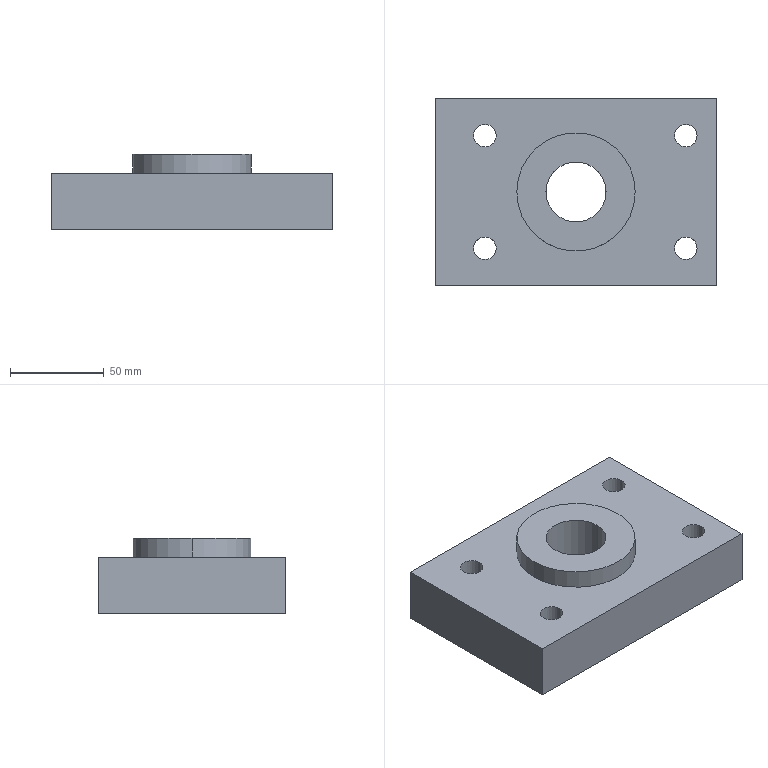Part | SolidWorks | features ICE 3, Extrusion 1 | 1 solid | 19 faces | box 150 x 100 x 40 mm | volume 435431 mm3 | cylinder 12 | plane 7 | commonest cylinder face diameters 12 x8 32 x2 63 x2
STEP:
#1=CARTESIAN_POINT('',(64.5,-30.,30.));
#2=VERTEX_POINT('',#1);
#3=CARTESIAN_POINT('',(52.5,-30.,30.));
#4=VERTEX_POINT('',#3);
#5=CARTESIAN_POINT('',(58.5,-30.,30.));
#6=DIRECTION('',(0.,0.,-1.));
#7=DIRECTION('',(-1.,0.,0.));
#8=AXIS2_PLACEMENT_3D('',#5,#6,#7);
#9=CIRCLE('',#8,6.);
#10=EDGE_CURVE('',#2,#4,#9,.T.);
#11=ORIENTED_EDGE('',*,*,#10,.F.);
#12=CARTESIAN_POINT('',(64.5,-30.,0.));
#13=VERTEX_POINT('',#12);
#14=CARTESIAN_POINT('',(64.5,-30.,40.));
#15=DIRECTION('',(0.,0.,-1.));
#16=VECTOR('',#15,1000.);
#17=LINE('',#14,#16);
#18=EDGE_CURVE('',#2,#13,#17,.T.);
#19=ORIENTED_EDGE('',*,*,#18,.T.);
#20=CARTESIAN_POINT('',(52.5,-30.,0.));
#21=VERTEX_POINT('',#20);
#22=CARTESIAN_POINT('',(58.5,-30.,0.));
#23=DIRECTION('',(0.,0.,-1.));
#24=DIRECTION('',(-1.,0.,0.));
#25=AXIS2_PLACEMENT_3D('',#22,#23,#24);
#26=CIRCLE('',#25,6.);
#27=EDGE_CURVE('',#13,#21,#26,.T.);
#28=ORIENTED_EDGE('',*,*,#27,.T.);
#29=CARTESIAN_POINT('',(52.5,-30.,40.));
#30=DIRECTION('',(0.,0.,-1.));
#31=VECTOR('',#30,1000.);
#32=LINE('',#29,#31);
#33=EDGE_CURVE('',#4,#21,#32,.T.);
#34=ORIENTED_EDGE('',*,*,#33,.F.);
#35=EDGE_LOOP('',(#11,#19,#28,#34));
#36=FACE_OUTER_BOUND('',#35,.T.);
#37=CARTESIAN_POINT('',(58.5,-30.,40.));
#38=DIRECTION('',(0.,0.,-1.));
#39=DIRECTION('',(-1.,0.,0.));
#40=AXIS2_PLACEMENT_3D('',#37,#38,#39);
#41=CYLINDRICAL_SURFACE('',#40,6.);
#42=ADVANCED_FACE('',(#36),#41,.F.);
#43=CARTESIAN_POINT('',(-42.5,-30.,30.));
#44=VERTEX_POINT('',#43);
#45=CARTESIAN_POINT('',(-54.5,-30.,30.));
#46=VERTEX_POINT('',#45);
#47=CARTESIAN_POINT('',(-48.5,-30.,30.));
#48=DIRECTION('',(0.,0.,-1.));
#49=DIRECTION('',(-1.,0.,0.));
#50=AXIS2_PLACEMENT_3D('',#47,#48,#49);
#51=CIRCLE('',#50,6.);
#52=EDGE_CURVE('',#44,#46,#51,.T.);
#53=ORIENTED_EDGE('',*,*,#52,.F.);
#54=CARTESIAN_POINT('',(-42.5,-30.,0.));
#55=VERTEX_POINT('',#54);
#56=CARTESIAN_POINT('',(-42.5,-30.,40.));
#57=DIRECTION('',(0.,0.,-1.));
#58=VECTOR('',#57,1000.);
#59=LINE('',#56,#58);
#60=EDGE_CURVE('',#44,#55,#59,.T.);
#61=ORIENTED_EDGE('',*,*,#60,.T.);
#62=CARTESIAN_POINT('',(-54.5,-30.,0.));
#63=VERTEX_POINT('',#62);
#64=CARTESIAN_POINT('',(-48.5,-30.,0.));
#65=DIRECTION('',(0.,0.,-1.));
#66=DIRECTION('',(-1.,0.,0.));
#67=AXIS2_PLACEMENT_3D('',#64,#65,#66);
#68=CIRCLE('',#67,6.);
#69=EDGE_CURVE('',#55,#63,#68,.T.);
#70=ORIENTED_EDGE('',*,*,#69,.T.);
#71=CARTESIAN_POINT('',(-54.5,-30.,40.));
#72=DIRECTION('',(0.,0.,-1.));
#73=VECTOR('',#72,1000.);
#74=LINE('',#71,#73);
#75=EDGE_CURVE('',#46,#63,#74,.T.);
#76=ORIENTED_EDGE('',*,*,#75,.F.);
#77=EDGE_LOOP('',(#53,#61,#70,#76));
#78=FACE_OUTER_BOUND('',#77,.T.);
#79=CARTESIAN_POINT('',(-48.5,-30.,40.));
#80=DIRECTION('',(0.,0.,-1.));
#81=DIRECTION('',(-1.,0.,0.));
#82=AXIS2_PLACEMENT_3D('',#79,#80,#81);
#83=CYLINDRICAL_SURFACE('',#82,6.);
#84=ADVANCED_FACE('',(#78),#83,.F.);
#85=CARTESIAN_POINT('',(-42.5,30.,30.));
#86=VERTEX_POINT('',#85);
#87=CARTESIAN_POINT('',(-54.5,30.,30.));
#88=VERTEX_POINT('',#87);
#89=CARTESIAN_POINT('',(-48.5,30.,30.));
#90=DIRECTION('',(0.,0.,-1.));
#91=DIRECTION('',(-1.,0.,0.));
#92=AXIS2_PLACEMENT_3D('',#89,#90,#91);
#93=CIRCLE('',#92,6.);
#94=EDGE_CURVE('',#86,#88,#93,.T.);
#95=ORIENTED_EDGE('',*,*,#94,.F.);
#96=CARTESIAN_POINT('',(-42.5,30.,0.));
#97=VERTEX_POINT('',#96);
#98=CARTESIAN_POINT('',(-42.5,30.,40.));
#99=DIRECTION('',(0.,0.,-1.));
#100=VECTOR('',#99,1000.);
#101=LINE('',#98,#100);
#102=EDGE_CURVE('',#86,#97,#101,.T.);
#103=ORIENTED_EDGE('',*,*,#102,.T.);
#104=CARTESIAN_POINT('',(-54.5,30.,0.));
#105=VERTEX_POINT('',#104);
#106=CARTESIAN_POINT('',(-48.5,30.,0.));
#107=DIRECTION('',(0.,0.,-1.));
#108=DIRECTION('',(-1.,0.,0.));
#109=AXIS2_PLACEMENT_3D('',#106,#107,#108);
#110=CIRCLE('',#109,6.);
#111=EDGE_CURVE('',#97,#105,#110,.T.);
#112=ORIENTED_EDGE('',*,*,#111,.T.);
#113=CARTESIAN_POINT('',(-54.5,30.,40.));
#114=DIRECTION('',(0.,0.,-1.));
#115=VECTOR('',#114,1000.);
#116=LINE('',#113,#115);
#117=EDGE_CURVE('',#88,#105,#116,.T.);
#118=ORIENTED_EDGE('',*,*,#117,.F.);
#119=EDGE_LOOP('',(#95,#103,#112,#118));
#120=FACE_OUTER_BOUND('',#119,.T.);
#121=CARTESIAN_POINT('',(-48.5,30.,40.));
#122=DIRECTION('',(0.,0.,-1.));
#123=DIRECTION('',(-1.,0.,0.));
#124=AXIS2_PLACEMENT_3D('',#121,#122,#123);
#125=CYLINDRICAL_SURFACE('',#124,6.);
#126=ADVANCED_FACE('',(#120),#125,.F.);
#127=CARTESIAN_POINT('',(64.5,30.,30.));
#128=VERTEX_POINT('',#127);
#129=CARTESIAN_POINT('',(52.5,30.,30.));
#130=VERTEX_POINT('',#129);
#131=CARTESIAN_POINT('',(58.5,30.,30.));
#132=DIRECTION('',(0.,0.,-1.));
#133=DIRECTION('',(-1.,0.,0.));
#134=AXIS2_PLACEMENT_3D('',#131,#132,#133);
#135=CIRCLE('',#134,6.);
#136=EDGE_CURVE('',#128,#130,#135,.T.);
#137=ORIENTED_EDGE('',*,*,#136,.F.);
#138=CARTESIAN_POINT('',(64.5,30.,0.));
#139=VERTEX_POINT('',#138);
#140=CARTESIAN_POINT('',(64.5,30.,40.));
#141=DIRECTION('',(0.,0.,-1.));
#142=VECTOR('',#141,1000.);
#143=LINE('',#140,#142);
#144=EDGE_CURVE('',#128,#139,#143,.T.);
#145=ORIENTED_EDGE('',*,*,#144,.T.);
#146=CARTESIAN_POINT('',(52.5,30.,0.));
#147=VERTEX_POINT('',#146);
#148=CARTESIAN_POINT('',(58.5,30.,0.));
#149=DIRECTION('',(0.,0.,-1.));
#150=DIRECTION('',(-1.,0.,0.));
#151=AXIS2_PLACEMENT_3D('',#148,#149,#150);
#152=CIRCLE('',#151,6.);
#153=EDGE_CURVE('',#139,#147,#152,.T.);
#154=ORIENTED_EDGE('',*,*,#153,.T.);
#155=CARTESIAN_POINT('',(52.5,30.,40.));
#156=DIRECTION('',(0.,0.,-1.));
#157=VECTOR('',#156,1000.);
#158=LINE('',#155,#157);
#159=EDGE_CURVE('',#130,#147,#158,.T.);
#160=ORIENTED_EDGE('',*,*,#159,.F.);
#161=EDGE_LOOP('',(#137,#145,#154,#160));
#162=FACE_OUTER_BOUND('',#161,.T.);
#163=CARTESIAN_POINT('',(58.5,30.,40.));
#164=DIRECTION('',(0.,0.,-1.));
#165=DIRECTION('',(-1.,0.,0.));
#166=AXIS2_PLACEMENT_3D('',#163,#164,#165);
#167=CYLINDRICAL_SURFACE('',#166,6.);
#168=ADVANCED_FACE('',(#162),#167,.F.);
#169=CARTESIAN_POINT('',(-16.,0.,40.));
#170=VERTEX_POINT('',#169);
#171=CARTESIAN_POINT('',(16.,0.,40.));
#172=VERTEX_POINT('',#171);
#173=CARTESIAN_POINT('',(0.,0.,40.));
#174=DIRECTION('',(0.,0.,1.));
#175=DIRECTION('',(1.,0.,0.));
#176=AXIS2_PLACEMENT_3D('',#173,#174,#175);
#177=CIRCLE('',#176,16.);
#178=EDGE_CURVE('',#170,#172,#177,.T.);
#179=ORIENTED_EDGE('',*,*,#178,.T.);
#180=CARTESIAN_POINT('',(16.,0.,0.));
#181=VERTEX_POINT('',#180);
#182=CARTESIAN_POINT('',(16.,0.,40.));
#183=DIRECTION('',(0.,0.,-1.));
#184=VECTOR('',#183,1000.);
#185=LINE('',#182,#184);
#186=EDGE_CURVE('',#172,#181,#185,.T.);
#187=ORIENTED_EDGE('',*,*,#186,.T.);
#188=CARTESIAN_POINT('',(-16.,0.,0.));
#189=VERTEX_POINT('',#188);
#190=CARTESIAN_POINT('',(0.,0.,0.));
#191=DIRECTION('',(0.,0.,1.));
#192=DIRECTION('',(1.,0.,0.));
#193=AXIS2_PLACEMENT_3D('',#190,#191,#192);
#194=CIRCLE('',#193,16.);
#195=EDGE_CURVE('',#189,#181,#194,.T.);
#196=ORIENTED_EDGE('',*,*,#195,.F.);
#197=CARTESIAN_POINT('',(-16.,0.,40.));
#198=DIRECTION('',(0.,0.,-1.));
#199=VECTOR('',#198,1000.);
#200=LINE('',#197,#199);
#201=EDGE_CURVE('',#170,#189,#200,.T.);
#202=ORIENTED_EDGE('',*,*,#201,.F.);
#203=EDGE_LOOP('',(#179,#187,#196,#202));
#204=FACE_OUTER_BOUND('',#203,.T.);
#205=CARTESIAN_POINT('',(0.,0.,40.));
#206=DIRECTION('',(0.,0.,-1.));
#207=DIRECTION('',(-1.,0.,0.));
#208=AXIS2_PLACEMENT_3D('',#205,#206,#207);
#209=CYLINDRICAL_SURFACE('',#208,16.);
#210=ADVANCED_FACE('',(#204),#209,.F.);
#211=CARTESIAN_POINT('',(31.5,0.,40.));
#212=VERTEX_POINT('',#211);
#213=CARTESIAN_POINT('',(-31.5,0.,40.));
#214=VERTEX_POINT('',#213);
#215=CARTESIAN_POINT('',(0.,0.,40.));
#216=DIRECTION('',(0.,0.,1.));
#217=DIRECTION('',(1.,0.,0.));
#218=AXIS2_PLACEMENT_3D('',#215,#216,#217);
#219=CIRCLE('',#218,31.5);
#220=EDGE_CURVE('',#212,#214,#219,.T.);
#221=ORIENTED_EDGE('',*,*,#220,.F.);
#222=CARTESIAN_POINT('',(31.5,0.,30.));
#223=VERTEX_POINT('',#222);
#224=CARTESIAN_POINT('',(31.5,0.,40.));
#225=DIRECTION('',(0.,0.,-1.));
#226=VECTOR('',#225,1000.);
#227=LINE('',#224,#226);
#228=EDGE_CURVE('',#212,#223,#227,.T.);
#229=ORIENTED_EDGE('',*,*,#228,.T.);
#230=CARTESIAN_POINT('',(-31.5,0.,30.));
#231=VERTEX_POINT('',#230);
#232=CARTESIAN_POINT('',(0.,0.,30.));
#233=DIRECTION('',(0.,0.,1.));
#234=DIRECTION('',(-1.,0.,0.));
#235=AXIS2_PLACEMENT_3D('',#232,#233,#234);
#236=CIRCLE('',#235,31.5);
#237=EDGE_CURVE('',#223,#231,#236,.T.);
#238=ORIENTED_EDGE('',*,*,#237,.T.);
#239=CARTESIAN_POINT('',(-31.5,0.,40.));
#240=DIRECTION('',(0.,0.,-1.));
#241=VECTOR('',#240,1000.);
#242=LINE('',#239,#241);
#243=EDGE_CURVE('',#214,#231,#242,.T.);
#244=ORIENTED_EDGE('',*,*,#243,.F.);
#245=EDGE_LOOP('',(#221,#229,#238,#244));
#246=FACE_OUTER_BOUND('',#245,.T.);
#247=CARTESIAN_POINT('',(0.,0.,40.));
#248=DIRECTION('',(0.,0.,-1.));
#249=DIRECTION('',(-1.,0.,0.));
#250=AXIS2_PLACEMENT_3D('',#247,#248,#249);
#251=CYLINDRICAL_SURFACE('',#250,31.5);
#252=ADVANCED_FACE('',(#246),#251,.T.);
#253=CARTESIAN_POINT('',(75.,-50.,0.));
#254=VERTEX_POINT('',#253);
#255=CARTESIAN_POINT('',(75.,50.,0.));
#256=VERTEX_POINT('',#255);
#257=CARTESIAN_POINT('',(75.,-50.,0.));
#258=DIRECTION('',(0.,1.,0.));
#259=VECTOR('',#258,1000.);
#260=LINE('',#257,#259);
#261=EDGE_CURVE('',#254,#256,#260,.T.);
#262=ORIENTED_EDGE('',*,*,#261,.T.);
#263=CARTESIAN_POINT('',(75.,50.,30.));
#264=VERTEX_POINT('',#263);
#265=CARTESIAN_POINT('',(75.,50.,30.));
#266=DIRECTION('',(0.,0.,-1.));
#267=VECTOR('',#266,1000.);
#268=LINE('',#265,#267);
#269=EDGE_CURVE('',#264,#256,#268,.T.);
#270=ORIENTED_EDGE('',*,*,#269,.F.);
#271=CARTESIAN_POINT('',(75.,-50.,30.));
#272=VERTEX_POINT('',#271);
#273=CARTESIAN_POINT('',(75.,-50.,30.));
#274=DIRECTION('',(0.,1.,0.));
#275=VECTOR('',#274,1000.);
#276=LINE('',#273,#275);
#277=EDGE_CURVE('',#272,#264,#276,.T.);
#278=ORIENTED_EDGE('',*,*,#277,.F.);
#279=CARTESIAN_POINT('',(75.,-50.,30.));
#280=DIRECTION('',(0.,0.,-1.));
#281=VECTOR('',#280,1000.);
#282=LINE('',#279,#281);
#283=EDGE_CURVE('',#272,#254,#282,.T.);
#284=ORIENTED_EDGE('',*,*,#283,.T.);
#285=EDGE_LOOP('',(#262,#270,#278,#284));
#286=FACE_OUTER_BOUND('',#285,.T.);
#287=CARTESIAN_POINT('',(75.,-50.,30.));
#288=DIRECTION('',(-1.,0.,0.));
#289=DIRECTION('',(0.,0.,1.));
#290=AXIS2_PLACEMENT_3D('',#287,#288,#289);
#291=PLANE('',#290);
#292=ADVANCED_FACE('',(#286),#291,.F.);
#293=CARTESIAN_POINT('',(-75.,50.,0.));
#294=VERTEX_POINT('',#293);
#295=CARTESIAN_POINT('',(-75.,50.,0.));
#296=DIRECTION('',(-1.,0.,0.));
#297=VECTOR('',#296,1000.);
#298=LINE('',#295,#297);
#299=EDGE_CURVE('',#256,#294,#298,.T.);
#300=ORIENTED_EDGE('',*,*,#299,.T.);
#301=CARTESIAN_POINT('',(-75.,50.,30.));
#302=VERTEX_POINT('',#301);
#303=CARTESIAN_POINT('',(-75.,50.,30.));
#304=DIRECTION('',(0.,0.,-1.));
#305=VECTOR('',#304,1000.);
#306=LINE('',#303,#305);
#307=EDGE_CURVE('',#302,#294,#306,.T.);
#308=ORIENTED_EDGE('',*,*,#307,.F.);
#309=CARTESIAN_POINT('',(-75.,50.,30.));
#310=DIRECTION('',(-1.,0.,0.));
#311=VECTOR('',#310,1000.);
#312=LINE('',#309,#311);
#313=EDGE_CURVE('',#264,#302,#312,.T.);
#314=ORIENTED_EDGE('',*,*,#313,.F.);
#315=ORIENTED_EDGE('',*,*,#269,.T.);
#316=EDGE_LOOP('',(#300,#308,#314,#315));
#317=FACE_OUTER_BOUND('',#316,.T.);
#318=CARTESIAN_POINT('',(-75.,50.,30.));
#319=DIRECTION('',(0.,-1.,0.));
#320=DIRECTION('',(0.,0.,-1.));
#321=AXIS2_PLACEMENT_3D('',#318,#319,#320);
#322=PLANE('',#321);
#323=ADVANCED_FACE('',(#317),#322,.F.);
#324=CARTESIAN_POINT('',(-75.,-50.,0.));
#325=VERTEX_POINT('',#324);
#326=CARTESIAN_POINT('',(-75.,-50.,0.));
#327=DIRECTION('',(0.,-1.,0.));
#328=VECTOR('',#327,1000.);
#329=LINE('',#326,#328);
#330=EDGE_CURVE('',#294,#325,#329,.T.);
#331=ORIENTED_EDGE('',*,*,#330,.T.);
#332=CARTESIAN_POINT('',(-75.,-50.,30.));
#333=VERTEX_POINT('',#332);
#334=CARTESIAN_POINT('',(-75.,-50.,30.));
#335=DIRECTION('',(0.,0.,-1.));
#336=VECTOR('',#335,1000.);
#337=LINE('',#334,#336);
#338=EDGE_CURVE('',#333,#325,#337,.T.);
#339=ORIENTED_EDGE('',*,*,#338,.F.);
#340=CARTESIAN_POINT('',(-75.,-50.,30.));
#341=DIRECTION('',(0.,-1.,0.));
#342=VECTOR('',#341,1000.);
#343=LINE('',#340,#342);
#344=EDGE_CURVE('',#302,#333,#343,.T.);
#345=ORIENTED_EDGE('',*,*,#344,.F.);
#346=ORIENTED_EDGE('',*,*,#307,.T.);
#347=EDGE_LOOP('',(#331,#339,#345,#346));
#348=FACE_OUTER_BOUND('',#347,.T.);
#349=CARTESIAN_POINT('',(-75.,-50.,30.));
#350=DIRECTION('',(1.,0.,0.));
#351=DIRECTION('',(0.,0.,-1.));
#352=AXIS2_PLACEMENT_3D('',#349,#350,#351);
#353=PLANE('',#352);
#354=ADVANCED_FACE('',(#348),#353,.F.);
#355=CARTESIAN_POINT('',(-75.,-50.,0.));
#356=DIRECTION('',(1.,0.,0.));
#357=VECTOR('',#356,1000.);
#358=LINE('',#355,#357);
#359=EDGE_CURVE('',#325,#254,#358,.T.);
#360=ORIENTED_EDGE('',*,*,#359,.T.);
#361=ORIENTED_EDGE('',*,*,#283,.F.);
#362=CARTESIAN_POINT('',(-75.,-50.,30.));
#363=DIRECTION('',(1.,0.,0.));
#364=VECTOR('',#363,1000.);
#365=LINE('',#362,#364);
#366=EDGE_CURVE('',#333,#272,#365,.T.);
#367=ORIENTED_EDGE('',*,*,#366,.F.);
#368=ORIENTED_EDGE('',*,*,#338,.T.);
#369=EDGE_LOOP('',(#360,#361,#367,#368));
#370=FACE_OUTER_BOUND('',#369,.T.);
#371=CARTESIAN_POINT('',(-75.,-50.,30.));
#372=DIRECTION('',(0.,1.,0.));
#373=DIRECTION('',(0.,0.,1.));
#374=AXIS2_PLACEMENT_3D('',#371,#372,#373);
#375=PLANE('',#374);
#376=ADVANCED_FACE('',(#370),#375,.F.);
#377=CARTESIAN_POINT('',(58.5,-30.,30.));
#378=DIRECTION('',(0.,0.,-1.));
#379=DIRECTION('',(-1.,0.,0.));
#380=AXIS2_PLACEMENT_3D('',#377,#378,#379);
#381=CIRCLE('',#380,6.);
#382=EDGE_CURVE('',#4,#2,#381,.T.);
#383=ORIENTED_EDGE('',*,*,#382,.T.);
#384=ORIENTED_EDGE('',*,*,#10,.T.);
#385=EDGE_LOOP('',(#383,#384));
#386=FACE_BOUND('',#385,.T.);
#387=CARTESIAN_POINT('',(-48.5,-30.,30.));
#388=DIRECTION('',(0.,0.,-1.));
#389=DIRECTION('',(-1.,0.,0.));
#390=AXIS2_PLACEMENT_3D('',#387,#388,#389);
#391=CIRCLE('',#390,6.);
#392=EDGE_CURVE('',#46,#44,#391,.T.);
#393=ORIENTED_EDGE('',*,*,#392,.T.);
#394=ORIENTED_EDGE('',*,*,#52,.T.);
#395=EDGE_LOOP('',(#393,#394));
#396=FACE_BOUND('',#395,.T.);
#397=CARTESIAN_POINT('',(-48.5,30.,30.));
#398=DIRECTION('',(0.,0.,-1.));
#399=DIRECTION('',(-1.,0.,0.));
#400=AXIS2_PLACEMENT_3D('',#397,#398,#399);
#401=CIRCLE('',#400,6.);
#402=EDGE_CURVE('',#88,#86,#401,.T.);
#403=ORIENTED_EDGE('',*,*,#402,.T.);
#404=ORIENTED_EDGE('',*,*,#94,.T.);
#405=EDGE_LOOP('',(#403,#404));
#406=FACE_BOUND('',#405,.T.);
#407=CARTESIAN_POINT('',(58.5,30.,30.));
#408=DIRECTION('',(0.,0.,-1.));
#409=DIRECTION('',(-1.,0.,0.));
#410=AXIS2_PLACEMENT_3D('',#407,#408,#409);
#411=CIRCLE('',#410,6.);
#412=EDGE_CURVE('',#130,#128,#411,.T.);
#413=ORIENTED_EDGE('',*,*,#412,.T.);
#414=ORIENTED_EDGE('',*,*,#136,.T.);
#415=EDGE_LOOP('',(#413,#414));
#416=FACE_BOUND('',#415,.T.);
#417=CARTESIAN_POINT('',(0.,0.,30.));
#418=DIRECTION('',(0.,0.,1.));
#419=DIRECTION('',(-1.,0.,0.));
#420=AXIS2_PLACEMENT_3D('',#417,#418,#419);
#421=CIRCLE('',#420,31.5);
#422=EDGE_CURVE('',#231,#223,#421,.T.);
#423=ORIENTED_EDGE('',*,*,#422,.F.);
#424=ORIENTED_EDGE('',*,*,#237,.F.);
#425=EDGE_LOOP('',(#423,#424));
#426=FACE_BOUND('',#425,.T.);
#427=ORIENTED_EDGE('',*,*,#277,.T.);
#428=ORIENTED_EDGE('',*,*,#313,.T.);
#429=ORIENTED_EDGE('',*,*,#344,.T.);
#430=ORIENTED_EDGE('',*,*,#366,.T.);
#431=EDGE_LOOP('',(#427,#428,#429,#430));
#432=FACE_OUTER_BOUND('',#431,.T.);
#433=CARTESIAN_POINT('',(0.,0.,30.));
#434=DIRECTION('',(0.,0.,-1.));
#435=DIRECTION('',(-1.,0.,0.));
#436=AXIS2_PLACEMENT_3D('',#433,#434,#435);
#437=PLANE('',#436);
#438=ADVANCED_FACE('',(#386,#396,#406,#416,#426,#432),#437,.F.);
#439=CARTESIAN_POINT('',(58.5,-30.,0.));
#440=DIRECTION('',(0.,0.,-1.));
#441=DIRECTION('',(-1.,0.,0.));
#442=AXIS2_PLACEMENT_3D('',#439,#440,#441);
#443=CIRCLE('',#442,6.);
#444=EDGE_CURVE('',#21,#13,#443,.T.);
#445=ORIENTED_EDGE('',*,*,#444,.F.);
#446=ORIENTED_EDGE('',*,*,#27,.F.);
#447=EDGE_LOOP('',(#445,#446));
#448=FACE_BOUND('',#447,.T.);
#449=CARTESIAN_POINT('',(-48.5,-30.,0.));
#450=DIRECTION('',(0.,0.,-1.));
#451=DIRECTION('',(-1.,0.,0.));
#452=AXIS2_PLACEMENT_3D('',#449,#450,#451);
#453=CIRCLE('',#452,6.);
#454=EDGE_CURVE('',#63,#55,#453,.T.);
#455=ORIENTED_EDGE('',*,*,#454,.F.);
#456=ORIENTED_EDGE('',*,*,#69,.F.);
#457=EDGE_LOOP('',(#455,#456));
#458=FACE_BOUND('',#457,.T.);
#459=CARTESIAN_POINT('',(-48.5,30.,0.));
#460=DIRECTION('',(0.,0.,-1.));
#461=DIRECTION('',(-1.,0.,0.));
#462=AXIS2_PLACEMENT_3D('',#459,#460,#461);
#463=CIRCLE('',#462,6.);
#464=EDGE_CURVE('',#105,#97,#463,.T.);
#465=ORIENTED_EDGE('',*,*,#464,.F.);
#466=ORIENTED_EDGE('',*,*,#111,.F.);
#467=EDGE_LOOP('',(#465,#466));
#468=FACE_BOUND('',#467,.T.);
#469=CARTESIAN_POINT('',(58.5,30.,0.));
#470=DIRECTION('',(0.,0.,-1.));
#471=DIRECTION('',(-1.,0.,0.));
#472=AXIS2_PLACEMENT_3D('',#469,#470,#471);
#473=CIRCLE('',#472,6.);
#474=EDGE_CURVE('',#147,#139,#473,.T.);
#475=ORIENTED_EDGE('',*,*,#474,.F.);
#476=ORIENTED_EDGE('',*,*,#153,.F.);
#477=EDGE_LOOP('',(#475,#476));
#478=FACE_BOUND('',#477,.T.);
#479=ORIENTED_EDGE('',*,*,#195,.T.);
#480=CARTESIAN_POINT('',(0.,0.,0.));
#481=DIRECTION('',(0.,0.,1.));
#482=DIRECTION('',(1.,0.,0.));
#483=AXIS2_PLACEMENT_3D('',#480,#481,#482);
#484=CIRCLE('',#483,16.);
#485=EDGE_CURVE('',#181,#189,#484,.T.);
#486=ORIENTED_EDGE('',*,*,#485,.T.);
#487=EDGE_LOOP('',(#479,#486));
#488=FACE_BOUND('',#487,.T.);
#489=ORIENTED_EDGE('',*,*,#261,.F.);
#490=ORIENTED_EDGE('',*,*,#359,.F.);
#491=ORIENTED_EDGE('',*,*,#330,.F.);
#492=ORIENTED_EDGE('',*,*,#299,.F.);
#493=EDGE_LOOP('',(#489,#490,#491,#492));
#494=FACE_OUTER_BOUND('',#493,.T.);
#495=CARTESIAN_POINT('',(0.,0.,0.));
#496=DIRECTION('',(0.,0.,-1.));
#497=DIRECTION('',(-1.,0.,0.));
#498=AXIS2_PLACEMENT_3D('',#495,#496,#497);
#499=PLANE('',#498);
#500=ADVANCED_FACE('',(#448,#458,#468,#478,#488,#494),#499,.T.);
#501=CARTESIAN_POINT('',(0.,0.,40.));
#502=DIRECTION('',(0.,0.,1.));
#503=DIRECTION('',(1.,0.,0.));
#504=AXIS2_PLACEMENT_3D('',#501,#502,#503);
#505=CIRCLE('',#504,31.5);
#506=EDGE_CURVE('',#214,#212,#505,.T.);
#507=ORIENTED_EDGE('',*,*,#506,.T.);
#508=ORIENTED_EDGE('',*,*,#220,.T.);
#509=EDGE_LOOP('',(#507,#508));
#510=FACE_OUTER_BOUND('',#509,.T.);
#511=ORIENTED_EDGE('',*,*,#178,.F.);
#512=CARTESIAN_POINT('',(0.,0.,40.));
#513=DIRECTION('',(0.,0.,1.));
#514=DIRECTION('',(1.,0.,0.));
#515=AXIS2_PLACEMENT_3D('',#512,#513,#514);
#516=CIRCLE('',#515,16.);
#517=EDGE_CURVE('',#172,#170,#516,.T.);
#518=ORIENTED_EDGE('',*,*,#517,.F.);
#519=EDGE_LOOP('',(#511,#518));
#520=FACE_BOUND('',#519,.T.);
#521=CARTESIAN_POINT('',(0.,0.,40.));
#522=DIRECTION('',(0.,0.,1.));
#523=DIRECTION('',(1.,0.,0.));
#524=AXIS2_PLACEMENT_3D('',#521,#522,#523);
#525=PLANE('',#524);
#526=ADVANCED_FACE('',(#510,#520),#525,.T.);
#527=ORIENTED_EDGE('',*,*,#228,.F.);
#528=ORIENTED_EDGE('',*,*,#506,.F.);
#529=ORIENTED_EDGE('',*,*,#243,.T.);
#530=ORIENTED_EDGE('',*,*,#422,.T.);
#531=EDGE_LOOP('',(#527,#528,#529,#530));
#532=FACE_OUTER_BOUND('',#531,.T.);
#533=CARTESIAN_POINT('',(0.,0.,40.));
#534=DIRECTION('',(0.,0.,-1.));
#535=DIRECTION('',(-1.,0.,0.));
#536=AXIS2_PLACEMENT_3D('',#533,#534,#535);
#537=CYLINDRICAL_SURFACE('',#536,31.5);
#538=ADVANCED_FACE('',(#532),#537,.T.);
#539=ORIENTED_EDGE('',*,*,#186,.F.);
#540=ORIENTED_EDGE('',*,*,#517,.T.);
#541=ORIENTED_EDGE('',*,*,#201,.T.);
#542=ORIENTED_EDGE('',*,*,#485,.F.);
#543=EDGE_LOOP('',(#539,#540,#541,#542));
#544=FACE_OUTER_BOUND('',#543,.T.);
#545=CARTESIAN_POINT('',(0.,0.,40.));
#546=DIRECTION('',(0.,0.,-1.));
#547=DIRECTION('',(-1.,0.,0.));
#548=AXIS2_PLACEMENT_3D('',#545,#546,#547);
#549=CYLINDRICAL_SURFACE('',#548,16.);
#550=ADVANCED_FACE('',(#544),#549,.F.);
#551=ORIENTED_EDGE('',*,*,#144,.F.);
#552=ORIENTED_EDGE('',*,*,#412,.F.);
#553=ORIENTED_EDGE('',*,*,#159,.T.);
#554=ORIENTED_EDGE('',*,*,#474,.T.);
#555=EDGE_LOOP('',(#551,#552,#553,#554));
#556=FACE_OUTER_BOUND('',#555,.T.);
#557=CARTESIAN_POINT('',(58.5,30.,40.));
#558=DIRECTION('',(0.,0.,-1.));
#559=DIRECTION('',(-1.,0.,0.));
#560=AXIS2_PLACEMENT_3D('',#557,#558,#559);
#561=CYLINDRICAL_SURFACE('',#560,6.);
#562=ADVANCED_FACE('',(#556),#561,.F.);
#563=ORIENTED_EDGE('',*,*,#102,.F.);
#564=ORIENTED_EDGE('',*,*,#402,.F.);
#565=ORIENTED_EDGE('',*,*,#117,.T.);
#566=ORIENTED_EDGE('',*,*,#464,.T.);
#567=EDGE_LOOP('',(#563,#564,#565,#566));
#568=FACE_OUTER_BOUND('',#567,.T.);
#569=CARTESIAN_POINT('',(-48.5,30.,40.));
#570=DIRECTION('',(0.,0.,-1.));
#571=DIRECTION('',(-1.,0.,0.));
#572=AXIS2_PLACEMENT_3D('',#569,#570,#571);
#573=CYLINDRICAL_SURFACE('',#572,6.);
#574=ADVANCED_FACE('',(#568),#573,.F.);
#575=ORIENTED_EDGE('',*,*,#60,.F.);
#576=ORIENTED_EDGE('',*,*,#392,.F.);
#577=ORIENTED_EDGE('',*,*,#75,.T.);
#578=ORIENTED_EDGE('',*,*,#454,.T.);
#579=EDGE_LOOP('',(#575,#576,#577,#578));
#580=FACE_OUTER_BOUND('',#579,.T.);
#581=CARTESIAN_POINT('',(-48.5,-30.,40.));
#582=DIRECTION('',(0.,0.,-1.));
#583=DIRECTION('',(-1.,0.,0.));
#584=AXIS2_PLACEMENT_3D('',#581,#582,#583);
#585=CYLINDRICAL_SURFACE('',#584,6.);
#586=ADVANCED_FACE('',(#580),#585,.F.);
#587=ORIENTED_EDGE('',*,*,#18,.F.);
#588=ORIENTED_EDGE('',*,*,#382,.F.);
#589=ORIENTED_EDGE('',*,*,#33,.T.);
#590=ORIENTED_EDGE('',*,*,#444,.T.);
#591=EDGE_LOOP('',(#587,#588,#589,#590));
#592=FACE_OUTER_BOUND('',#591,.T.);
#593=CARTESIAN_POINT('',(58.5,-30.,40.));
#594=DIRECTION('',(0.,0.,-1.));
#595=DIRECTION('',(-1.,0.,0.));
#596=AXIS2_PLACEMENT_3D('',#593,#594,#595);
#597=CYLINDRICAL_SURFACE('',#596,6.);
#598=ADVANCED_FACE('',(#592),#597,.F.);
#599=CLOSED_SHELL('',(#42,#84,#126,#168,#210,#252,#292,#323,#354,#376,#438,#500,#526,#538,#550,#562,#574,#586,#598));
#600=MANIFOLD_SOLID_BREP('',#599);
#601=CARTESIAN_POINT('',(0.,0.,0.));
#602=DIRECTION('',(0.,0.,1.));
#603=DIRECTION('',(1.,0.,0.));
#604=AXIS2_PLACEMENT_3D('',#601,#602,#603);
#605=(LENGTH_UNIT()NAMED_UNIT(*)SI_UNIT(.MILLI.,.METRE.));
#606=UNCERTAINTY_MEASURE_WITH_UNIT(LENGTH_MEASURE(0.00001),#605,'','');
#607=(NAMED_UNIT(*)PLANE_ANGLE_UNIT()SI_UNIT($,.RADIAN.));
#608=(NAMED_UNIT(*)SI_UNIT($,.STERADIAN.)SOLID_ANGLE_UNIT());
#609=(GEOMETRIC_REPRESENTATION_CONTEXT(3)GLOBAL_UNCERTAINTY_ASSIGNED_CONTEXT((#606))GLOBAL_UNIT_ASSIGNED_CONTEXT((#605,#607,#608))REPRESENTATION_CONTEXT('',''));
#610=ADVANCED_BREP_SHAPE_REPRESENTATION('',(#600,#604),#609);